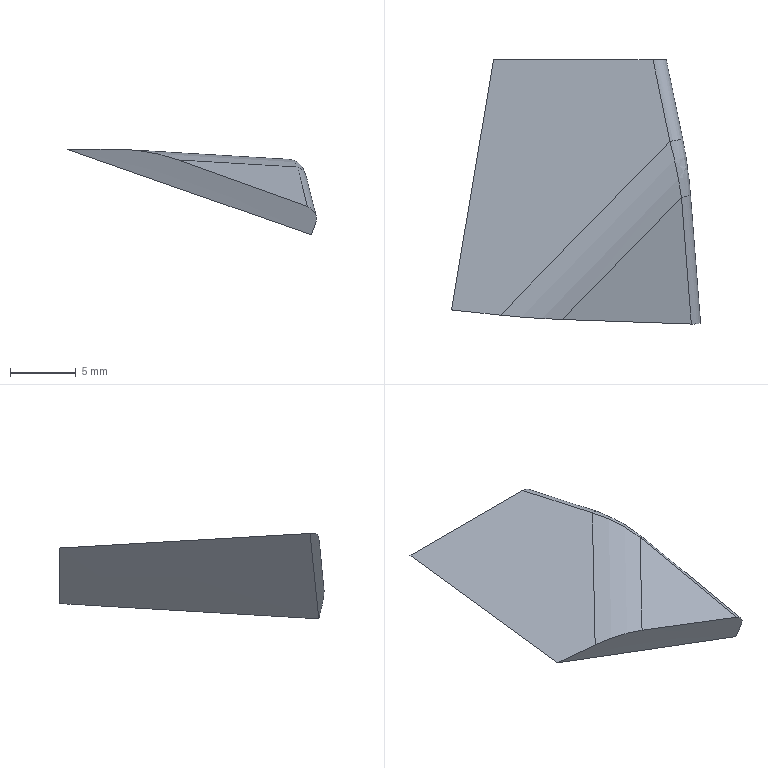Part | STEP file | solid 27 | 1 solid | 10 faces | box 18.904 x 20.052 x 6.503 mm | volume 764.337 mm3 | plane 4 | cylinder 3 | spline 2 | other 1 | commonest cylinder face diameters 2 x2 16 x1